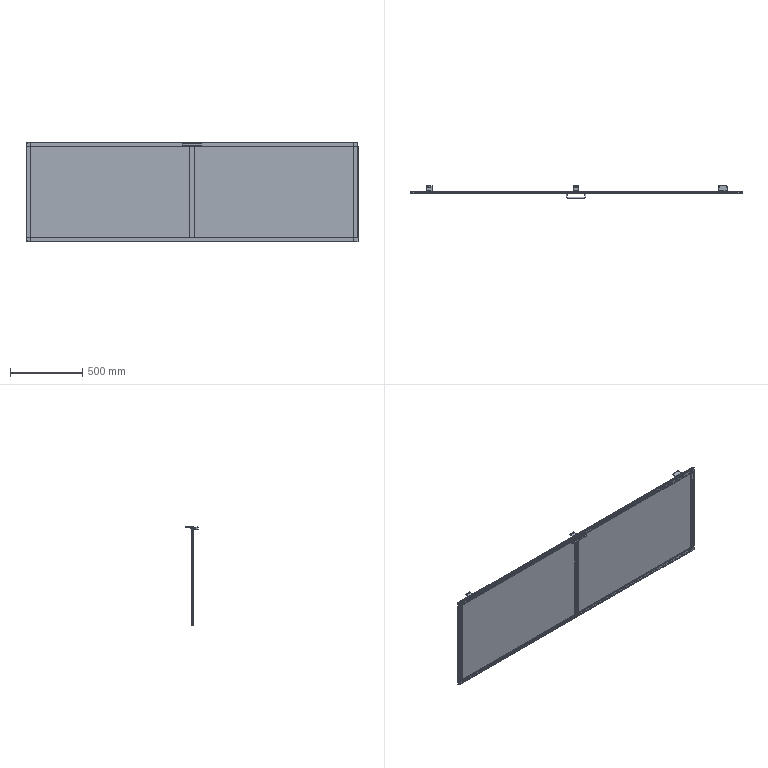Part | 39 solids | 1337 faces | box 2296 x 84 x 690 mm | volume 8839553 mm3 | plane 792 | cylinder 369 | cone 120 | spline 56 | commonest cylinder face diameters 5 x67 11 x52 1 x42 4.5 x40 3.3 x28 2 x20